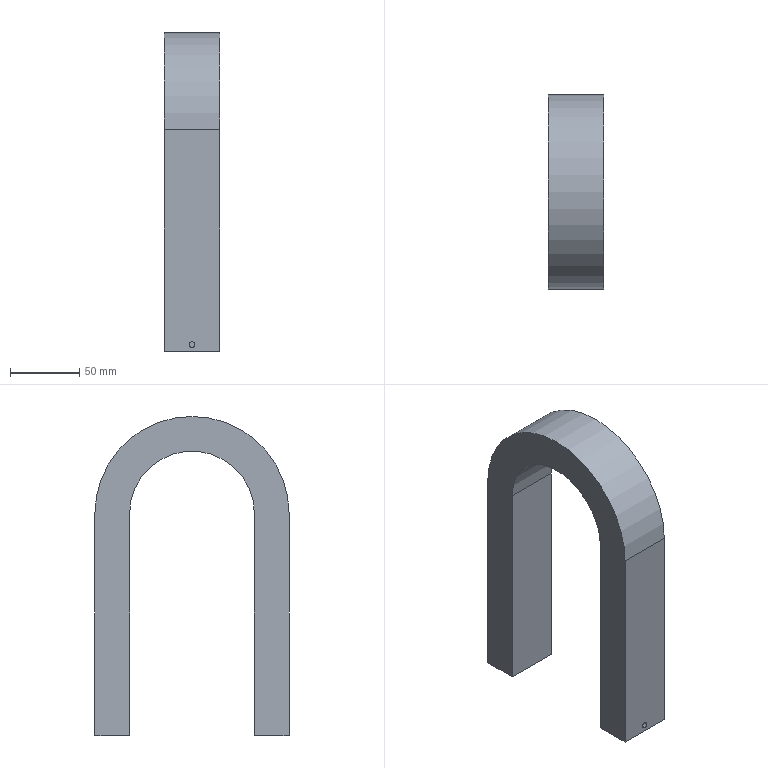Part | STEP file | material-separating mechanism drag chain | 1 solid | 12 faces | box 40 x 140 x 230 mm | volume 500295 mm3 | plane 8 | cylinder 4 | commonest cylinder face diameters 4.2 x2 90 x1 140 x1
STEP:
#1=CARTESIAN_POINT('',(0.,0.,0.));
#2=DIRECTION('',(0.,0.,1.));
#3=DIRECTION('',(1.,0.,0.));
#4=AXIS2_PLACEMENT_3D('',#1,#2,#3);
#5=CARTESIAN_POINT('',(5.,0.,7.1));
#6=VERTEX_POINT('',#5);
#7=CARTESIAN_POINT('',(5.,25.,7.1));
#8=VERTEX_POINT('',#7);
#9=CARTESIAN_POINT('',(5.,25.,7.1));
#10=DIRECTION('',(0.,1.,0.));
#11=VECTOR('',#10,1.);
#12=LINE('',#9,#11);
#13=CARTESIAN_POINT('',(5.,25.,5.));
#14=DIRECTION('',(0.,1.,0.));
#15=DIRECTION('',(0.,0.,1.));
#16=AXIS2_PLACEMENT_3D('',#13,#14,#15);
#17=CYLINDRICAL_SURFACE('',#16,2.1);
#18=CARTESIAN_POINT('',(6.283,0.));
#19=DIRECTION('',(0.,1.));
#20=VECTOR('',#19,1.);
#21=LINE('',#18,#20);
#22=(GEOMETRIC_REPRESENTATION_CONTEXT(2)PARAMETRIC_REPRESENTATION_CONTEXT()REPRESENTATION_CONTEXT('',''));
#23=DEFINITIONAL_REPRESENTATION('',(#21),#22);
#24=PCURVE('',#17,#23);
#25=CARTESIAN_POINT('',(5.,25.,5.));
#26=DIRECTION('',(0.,1.,0.));
#27=DIRECTION('',(0.,0.,1.));
#28=AXIS2_PLACEMENT_3D('',#25,#26,#27);
#29=CYLINDRICAL_SURFACE('',#28,2.1);
#30=CARTESIAN_POINT('',(0.,0.));
#31=DIRECTION('',(0.,1.));
#32=VECTOR('',#31,1.);
#33=LINE('',#30,#32);
#34=(GEOMETRIC_REPRESENTATION_CONTEXT(2)PARAMETRIC_REPRESENTATION_CONTEXT()REPRESENTATION_CONTEXT('',''));
#35=DEFINITIONAL_REPRESENTATION('',(#33),#34);
#36=PCURVE('',#29,#35);
#37=SURFACE_CURVE('',#12,(#24,#36),.PCURVE_S1.);
#38=EDGE_CURVE('',#6,#8,#37,.T.);
#39=ORIENTED_EDGE('',*,*,#38,.T.);
#40=CARTESIAN_POINT('',(5.,25.,2.9));
#41=VERTEX_POINT('',#40);
#42=CARTESIAN_POINT('',(5.,25.,5.));
#43=DIRECTION('',(0.,1.,0.));
#44=DIRECTION('',(0.,0.,1.));
#45=AXIS2_PLACEMENT_3D('',#42,#43,#44);
#46=CIRCLE('',#45,2.1);
#47=CARTESIAN_POINT('',(0.,0.));
#48=DIRECTION('',(1.,0.));
#49=VECTOR('',#48,1.);
#50=LINE('',#47,#49);
#51=(GEOMETRIC_REPRESENTATION_CONTEXT(2)PARAMETRIC_REPRESENTATION_CONTEXT()REPRESENTATION_CONTEXT('',''));
#52=DEFINITIONAL_REPRESENTATION('',(#50),#51);
#53=PCURVE('',#17,#52);
#54=CARTESIAN_POINT('',(-15.,25.,0.));
#55=DIRECTION('',(0.,1.,0.));
#56=DIRECTION('',(0.,0.,1.));
#57=AXIS2_PLACEMENT_3D('',#54,#55,#56);
#58=PLANE('',#57);
#59=CARTESIAN_POINT('',(5.,20.));
#60=DIRECTION('',(1.,0.));
#61=AXIS2_PLACEMENT_2D('',#59,#60);
#62=CIRCLE('',#61,2.1);
#63=(GEOMETRIC_REPRESENTATION_CONTEXT(2)PARAMETRIC_REPRESENTATION_CONTEXT()REPRESENTATION_CONTEXT('',''));
#64=DEFINITIONAL_REPRESENTATION('',(#62),#63);
#65=PCURVE('',#58,#64);
#66=SURFACE_CURVE('',#46,(#53,#65),.PCURVE_S1.);
#67=EDGE_CURVE('',#41,#8,#66,.T.);
#68=ORIENTED_EDGE('',*,*,#67,.F.);
#69=CARTESIAN_POINT('',(5.,0.,2.9));
#70=VERTEX_POINT('',#69);
#71=CARTESIAN_POINT('',(5.,25.,2.9));
#72=DIRECTION('',(0.,1.,0.));
#73=VECTOR('',#72,1.);
#74=LINE('',#71,#73);
#75=CARTESIAN_POINT('',(3.142,0.));
#76=DIRECTION('',(0.,1.));
#77=VECTOR('',#76,1.);
#78=LINE('',#75,#77);
#79=(GEOMETRIC_REPRESENTATION_CONTEXT(2)PARAMETRIC_REPRESENTATION_CONTEXT()REPRESENTATION_CONTEXT('',''));
#80=DEFINITIONAL_REPRESENTATION('',(#78),#79);
#81=PCURVE('',#17,#80);
#82=CARTESIAN_POINT('',(3.142,0.));
#83=DIRECTION('',(0.,1.));
#84=VECTOR('',#83,1.);
#85=LINE('',#82,#84);
#86=(GEOMETRIC_REPRESENTATION_CONTEXT(2)PARAMETRIC_REPRESENTATION_CONTEXT()REPRESENTATION_CONTEXT('',''));
#87=DEFINITIONAL_REPRESENTATION('',(#85),#86);
#88=PCURVE('',#29,#87);
#89=SURFACE_CURVE('',#74,(#81,#88),.PCURVE_S1.);
#90=EDGE_CURVE('',#70,#41,#89,.T.);
#91=ORIENTED_EDGE('',*,*,#90,.F.);
#92=CARTESIAN_POINT('',(5.,0.,5.));
#93=DIRECTION('',(0.,1.,0.));
#94=DIRECTION('',(0.,0.,1.));
#95=AXIS2_PLACEMENT_3D('',#92,#93,#94);
#96=CIRCLE('',#95,2.1);
#97=CARTESIAN_POINT('',(0.,-25.));
#98=DIRECTION('',(1.,0.));
#99=VECTOR('',#98,1.);
#100=LINE('',#97,#99);
#101=(GEOMETRIC_REPRESENTATION_CONTEXT(2)PARAMETRIC_REPRESENTATION_CONTEXT()REPRESENTATION_CONTEXT('',''));
#102=DEFINITIONAL_REPRESENTATION('',(#100),#101);
#103=PCURVE('',#17,#102);
#104=CARTESIAN_POINT('',(-15.,0.,0.));
#105=DIRECTION('',(0.,-1.,0.));
#106=DIRECTION('',(0.,0.,-1.));
#107=AXIS2_PLACEMENT_3D('',#104,#105,#106);
#108=PLANE('',#107);
#109=CARTESIAN_POINT('',(-7.1,20.));
#110=CARTESIAN_POINT('',(-7.1,23.637));
#111=CARTESIAN_POINT('',(-3.95,21.819));
#112=CARTESIAN_POINT('',(-0.8,20.));
#113=CARTESIAN_POINT('',(-3.95,18.181));
#114=CARTESIAN_POINT('',(-7.1,16.363));
#115=CARTESIAN_POINT('',(-7.1,20.));
#116=(BOUNDED_CURVE()B_SPLINE_CURVE(2,(#109,#110,#111,#112,#113,#114,#115),.UNSPECIFIED.,.T.,.F.)B_SPLINE_CURVE_WITH_KNOTS((1,2,2,2,2,1),(-2.094,0.,2.094,4.189,6.283,8.378),.UNSPECIFIED.)CURVE()GEOMETRIC_REPRESENTATION_ITEM()RATIONAL_B_SPLINE_CURVE((1.,0.5,1.,0.5,1.,0.5,1.))REPRESENTATION_ITEM(''));
#117=(GEOMETRIC_REPRESENTATION_CONTEXT(2)PARAMETRIC_REPRESENTATION_CONTEXT()REPRESENTATION_CONTEXT('',''));
#118=DEFINITIONAL_REPRESENTATION('',(#116),#117);
#119=PCURVE('',#108,#118);
#120=SURFACE_CURVE('',#96,(#103,#119),.PCURVE_S1.);
#121=EDGE_CURVE('',#70,#6,#120,.T.);
#122=ORIENTED_EDGE('',*,*,#121,.T.);
#123=EDGE_LOOP('',(#39,#68,#91,#122));
#124=FACE_BOUND('',#123,.F.);
#125=ADVANCED_FACE('',(#124),#17,.F.);
#126=CARTESIAN_POINT('',(-15.,0.,160.));
#127=VERTEX_POINT('',#126);
#128=CARTESIAN_POINT('',(25.,0.,160.));
#129=VERTEX_POINT('',#128);
#130=CARTESIAN_POINT('',(-15.,0.,160.));
#131=DIRECTION('',(1.,0.,0.));
#132=VECTOR('',#131,1.);
#133=LINE('',#130,#132);
#134=CARTESIAN_POINT('',(-15.,70.,160.));
#135=DIRECTION('',(1.,0.,0.));
#136=DIRECTION('',(0.,0.,-1.));
#137=AXIS2_PLACEMENT_3D('',#134,#135,#136);
#138=CYLINDRICAL_SURFACE('',#137,70.);
#139=CARTESIAN_POINT('',(4.712,0.));
#140=DIRECTION('',(0.,1.));
#141=VECTOR('',#140,1.);
#142=LINE('',#139,#141);
#143=(GEOMETRIC_REPRESENTATION_CONTEXT(2)PARAMETRIC_REPRESENTATION_CONTEXT()REPRESENTATION_CONTEXT('',''));
#144=DEFINITIONAL_REPRESENTATION('',(#142),#143);
#145=PCURVE('',#138,#144);
#146=CARTESIAN_POINT('',(-160.,0.));
#147=DIRECTION('',(0.,1.));
#148=VECTOR('',#147,1.);
#149=LINE('',#146,#148);
#150=(GEOMETRIC_REPRESENTATION_CONTEXT(2)PARAMETRIC_REPRESENTATION_CONTEXT()REPRESENTATION_CONTEXT('',''));
#151=DEFINITIONAL_REPRESENTATION('',(#149),#150);
#152=PCURVE('',#108,#151);
#153=SURFACE_CURVE('',#133,(#145,#152),.PCURVE_S1.);
#154=EDGE_CURVE('',#127,#129,#153,.T.);
#155=ORIENTED_EDGE('',*,*,#154,.T.);
#156=CARTESIAN_POINT('',(25.,140.,160.));
#157=VERTEX_POINT('',#156);
#158=CARTESIAN_POINT('',(25.,70.,160.));
#159=DIRECTION('',(1.,0.,0.));
#160=DIRECTION('',(0.,0.,-1.));
#161=AXIS2_PLACEMENT_3D('',#158,#159,#160);
#162=CIRCLE('',#161,70.);
#163=CARTESIAN_POINT('',(0.,40.));
#164=DIRECTION('',(1.,0.));
#165=VECTOR('',#164,1.);
#166=LINE('',#163,#165);
#167=(GEOMETRIC_REPRESENTATION_CONTEXT(2)PARAMETRIC_REPRESENTATION_CONTEXT()REPRESENTATION_CONTEXT('',''));
#168=DEFINITIONAL_REPRESENTATION('',(#166),#167);
#169=PCURVE('',#138,#168);
#170=CARTESIAN_POINT('',(25.,70.,160.));
#171=DIRECTION('',(1.,0.,0.));
#172=DIRECTION('',(0.,0.,-1.));
#173=AXIS2_PLACEMENT_3D('',#170,#171,#172);
#174=PLANE('',#173);
#175=CARTESIAN_POINT('',(0.,0.));
#176=DIRECTION('',(1.,0.));
#177=AXIS2_PLACEMENT_2D('',#175,#176);
#178=CIRCLE('',#177,70.);
#179=(GEOMETRIC_REPRESENTATION_CONTEXT(2)PARAMETRIC_REPRESENTATION_CONTEXT()REPRESENTATION_CONTEXT('',''));
#180=DEFINITIONAL_REPRESENTATION('',(#178),#179);
#181=PCURVE('',#174,#180);
#182=SURFACE_CURVE('',#162,(#169,#181),.PCURVE_S1.);
#183=EDGE_CURVE('',#157,#129,#182,.T.);
#184=ORIENTED_EDGE('',*,*,#183,.F.);
#185=CARTESIAN_POINT('',(-15.,140.,160.));
#186=VERTEX_POINT('',#185);
#187=CARTESIAN_POINT('',(-15.,140.,160.));
#188=DIRECTION('',(1.,0.,0.));
#189=VECTOR('',#188,1.);
#190=LINE('',#187,#189);
#191=CARTESIAN_POINT('',(1.571,0.));
#192=DIRECTION('',(0.,1.));
#193=VECTOR('',#192,1.);
#194=LINE('',#191,#193);
#195=(GEOMETRIC_REPRESENTATION_CONTEXT(2)PARAMETRIC_REPRESENTATION_CONTEXT()REPRESENTATION_CONTEXT('',''));
#196=DEFINITIONAL_REPRESENTATION('',(#194),#195);
#197=PCURVE('',#138,#196);
#198=CARTESIAN_POINT('',(-15.,140.,0.));
#199=DIRECTION('',(0.,1.,0.));
#200=DIRECTION('',(0.,0.,1.));
#201=AXIS2_PLACEMENT_3D('',#198,#199,#200);
#202=PLANE('',#201);
#203=CARTESIAN_POINT('',(160.,0.));
#204=DIRECTION('',(0.,1.));
#205=VECTOR('',#204,1.);
#206=LINE('',#203,#205);
#207=(GEOMETRIC_REPRESENTATION_CONTEXT(2)PARAMETRIC_REPRESENTATION_CONTEXT()REPRESENTATION_CONTEXT('',''));
#208=DEFINITIONAL_REPRESENTATION('',(#206),#207);
#209=PCURVE('',#202,#208);
#210=SURFACE_CURVE('',#190,(#197,#209),.PCURVE_S1.);
#211=EDGE_CURVE('',#186,#157,#210,.T.);
#212=ORIENTED_EDGE('',*,*,#211,.F.);
#213=CARTESIAN_POINT('',(-15.,70.,160.));
#214=DIRECTION('',(1.,0.,0.));
#215=DIRECTION('',(0.,0.,-1.));
#216=AXIS2_PLACEMENT_3D('',#213,#214,#215);
#217=CIRCLE('',#216,70.);
#218=CARTESIAN_POINT('',(0.,0.));
#219=DIRECTION('',(1.,0.));
#220=VECTOR('',#219,1.);
#221=LINE('',#218,#220);
#222=(GEOMETRIC_REPRESENTATION_CONTEXT(2)PARAMETRIC_REPRESENTATION_CONTEXT()REPRESENTATION_CONTEXT('',''));
#223=DEFINITIONAL_REPRESENTATION('',(#221),#222);
#224=PCURVE('',#138,#223);
#225=CARTESIAN_POINT('',(-15.,70.,160.));
#226=DIRECTION('',(1.,0.,0.));
#227=DIRECTION('',(0.,0.,-1.));
#228=AXIS2_PLACEMENT_3D('',#225,#226,#227);
#229=PLANE('',#228);
#230=CARTESIAN_POINT('',(0.,0.));
#231=DIRECTION('',(1.,0.));
#232=AXIS2_PLACEMENT_2D('',#230,#231);
#233=CIRCLE('',#232,70.);
#234=(GEOMETRIC_REPRESENTATION_CONTEXT(2)PARAMETRIC_REPRESENTATION_CONTEXT()REPRESENTATION_CONTEXT('',''));
#235=DEFINITIONAL_REPRESENTATION('',(#233),#234);
#236=PCURVE('',#229,#235);
#237=SURFACE_CURVE('',#217,(#224,#236),.PCURVE_S1.);
#238=EDGE_CURVE('',#186,#127,#237,.T.);
#239=ORIENTED_EDGE('',*,*,#238,.T.);
#240=EDGE_LOOP('',(#155,#184,#212,#239));
#241=FACE_BOUND('',#240,.T.);
#242=ADVANCED_FACE('',(#241),#138,.T.);
#243=ORIENTED_EDGE('',*,*,#211,.T.);
#244=CARTESIAN_POINT('',(25.,140.,0.));
#245=VERTEX_POINT('',#244);
#246=CARTESIAN_POINT('',(25.,140.,0.));
#247=DIRECTION('',(0.,0.,1.));
#248=VECTOR('',#247,1.);
#249=LINE('',#246,#248);
#250=CARTESIAN_POINT('',(0.,40.));
#251=DIRECTION('',(1.,0.));
#252=VECTOR('',#251,1.);
#253=LINE('',#250,#252);
#254=(GEOMETRIC_REPRESENTATION_CONTEXT(2)PARAMETRIC_REPRESENTATION_CONTEXT()REPRESENTATION_CONTEXT('',''));
#255=DEFINITIONAL_REPRESENTATION('',(#253),#254);
#256=PCURVE('',#202,#255);
#257=CARTESIAN_POINT('',(160.,70.));
#258=DIRECTION('',(-1.,0.));
#259=VECTOR('',#258,1.);
#260=LINE('',#257,#259);
#261=(GEOMETRIC_REPRESENTATION_CONTEXT(2)PARAMETRIC_REPRESENTATION_CONTEXT()REPRESENTATION_CONTEXT('',''));
#262=DEFINITIONAL_REPRESENTATION('',(#260),#261);
#263=PCURVE('',#174,#262);
#264=SURFACE_CURVE('',#249,(#256,#263),.PCURVE_S1.);
#265=EDGE_CURVE('',#245,#157,#264,.T.);
#266=ORIENTED_EDGE('',*,*,#265,.F.);
#267=CARTESIAN_POINT('',(-15.,140.,0.));
#268=VERTEX_POINT('',#267);
#269=CARTESIAN_POINT('',(-15.,140.,0.));
#270=DIRECTION('',(1.,0.,0.));
#271=VECTOR('',#270,1.);
#272=LINE('',#269,#271);
#273=CARTESIAN_POINT('',(0.,0.));
#274=DIRECTION('',(0.,1.));
#275=VECTOR('',#274,1.);
#276=LINE('',#273,#275);
#277=(GEOMETRIC_REPRESENTATION_CONTEXT(2)PARAMETRIC_REPRESENTATION_CONTEXT()REPRESENTATION_CONTEXT('',''));
#278=DEFINITIONAL_REPRESENTATION('',(#276),#277);
#279=PCURVE('',#202,#278);
#280=CARTESIAN_POINT('',(-15.,140.,0.));
#281=DIRECTION('',(0.,0.,-1.));
#282=DIRECTION('',(0.,1.,0.));
#283=AXIS2_PLACEMENT_3D('',#280,#281,#282);
#284=PLANE('',#283);
#285=CARTESIAN_POINT('',(0.,0.));
#286=DIRECTION('',(0.,1.));
#287=VECTOR('',#286,1.);
#288=LINE('',#285,#287);
#289=(GEOMETRIC_REPRESENTATION_CONTEXT(2)PARAMETRIC_REPRESENTATION_CONTEXT()REPRESENTATION_CONTEXT('',''));
#290=DEFINITIONAL_REPRESENTATION('',(#288),#289);
#291=PCURVE('',#284,#290);
#292=SURFACE_CURVE('',#272,(#279,#291),.PCURVE_S1.);
#293=EDGE_CURVE('',#268,#245,#292,.T.);
#294=ORIENTED_EDGE('',*,*,#293,.F.);
#295=CARTESIAN_POINT('',(-15.,140.,0.));
#296=DIRECTION('',(0.,0.,1.));
#297=VECTOR('',#296,1.);
#298=LINE('',#295,#297);
#299=CARTESIAN_POINT('',(0.,0.));
#300=DIRECTION('',(1.,0.));
#301=VECTOR('',#300,1.);
#302=LINE('',#299,#301);
#303=(GEOMETRIC_REPRESENTATION_CONTEXT(2)PARAMETRIC_REPRESENTATION_CONTEXT()REPRESENTATION_CONTEXT('',''));
#304=DEFINITIONAL_REPRESENTATION('',(#302),#303);
#305=PCURVE('',#202,#304);
#306=CARTESIAN_POINT('',(160.,70.));
#307=DIRECTION('',(-1.,0.));
#308=VECTOR('',#307,1.);
#309=LINE('',#306,#308);
#310=(GEOMETRIC_REPRESENTATION_CONTEXT(2)PARAMETRIC_REPRESENTATION_CONTEXT()REPRESENTATION_CONTEXT('',''));
#311=DEFINITIONAL_REPRESENTATION('',(#309),#310);
#312=PCURVE('',#229,#311);
#313=SURFACE_CURVE('',#298,(#305,#312),.PCURVE_S1.);
#314=EDGE_CURVE('',#268,#186,#313,.T.);
#315=ORIENTED_EDGE('',*,*,#314,.T.);
#316=EDGE_LOOP('',(#243,#266,#294,#315));
#317=FACE_BOUND('',#316,.T.);
#318=ADVANCED_FACE('',(#317),#202,.T.);
#319=ORIENTED_EDGE('',*,*,#293,.T.);
#320=CARTESIAN_POINT('',(25.,115.,0.));
#321=VERTEX_POINT('',#320);
#322=CARTESIAN_POINT('',(25.,140.,0.));
#323=DIRECTION('',(0.,1.,0.));
#324=VECTOR('',#323,1.);
#325=LINE('',#322,#324);
#326=CARTESIAN_POINT('',(0.,40.));
#327=DIRECTION('',(1.,0.));
#328=VECTOR('',#327,1.);
#329=LINE('',#326,#328);
#330=(GEOMETRIC_REPRESENTATION_CONTEXT(2)PARAMETRIC_REPRESENTATION_CONTEXT()REPRESENTATION_CONTEXT('',''));
#331=DEFINITIONAL_REPRESENTATION('',(#329),#330);
#332=PCURVE('',#284,#331);
#333=CARTESIAN_POINT('',(160.,70.));
#334=DIRECTION('',(0.,1.));
#335=VECTOR('',#334,1.);
#336=LINE('',#333,#335);
#337=(GEOMETRIC_REPRESENTATION_CONTEXT(2)PARAMETRIC_REPRESENTATION_CONTEXT()REPRESENTATION_CONTEXT('',''));
#338=DEFINITIONAL_REPRESENTATION('',(#336),#337);
#339=PCURVE('',#174,#338);
#340=SURFACE_CURVE('',#325,(#332,#339),.PCURVE_S1.);
#341=EDGE_CURVE('',#321,#245,#340,.T.);
#342=ORIENTED_EDGE('',*,*,#341,.F.);
#343=CARTESIAN_POINT('',(-15.,115.,0.));
#344=VERTEX_POINT('',#343);
#345=CARTESIAN_POINT('',(-15.,115.,0.));
#346=DIRECTION('',(1.,0.,0.));
#347=VECTOR('',#346,1.);
#348=LINE('',#345,#347);
#349=CARTESIAN_POINT('',(-25.,0.));
#350=DIRECTION('',(0.,1.));
#351=VECTOR('',#350,1.);
#352=LINE('',#349,#351);
#353=(GEOMETRIC_REPRESENTATION_CONTEXT(2)PARAMETRIC_REPRESENTATION_CONTEXT()REPRESENTATION_CONTEXT('',''));
#354=DEFINITIONAL_REPRESENTATION('',(#352),#353);
#355=PCURVE('',#284,#354);
#356=CARTESIAN_POINT('',(-15.,115.,0.));
#357=DIRECTION('',(0.,-1.,0.));
#358=DIRECTION('',(0.,0.,-1.));
#359=AXIS2_PLACEMENT_3D('',#356,#357,#358);
#360=PLANE('',#359);
#361=CARTESIAN_POINT('',(0.,0.));
#362=DIRECTION('',(0.,1.));
#363=VECTOR('',#362,1.);
#364=LINE('',#361,#363);
#365=(GEOMETRIC_REPRESENTATION_CONTEXT(2)PARAMETRIC_REPRESENTATION_CONTEXT()REPRESENTATION_CONTEXT('',''));
#366=DEFINITIONAL_REPRESENTATION('',(#364),#365);
#367=PCURVE('',#360,#366);
#368=SURFACE_CURVE('',#348,(#355,#367),.PCURVE_S1.);
#369=EDGE_CURVE('',#344,#321,#368,.T.);
#370=ORIENTED_EDGE('',*,*,#369,.F.);
#371=CARTESIAN_POINT('',(-15.,140.,0.));
#372=DIRECTION('',(0.,1.,0.));
#373=VECTOR('',#372,1.);
#374=LINE('',#371,#373);
#375=CARTESIAN_POINT('',(0.,0.));
#376=DIRECTION('',(1.,0.));
#377=VECTOR('',#376,1.);
#378=LINE('',#375,#377);
#379=(GEOMETRIC_REPRESENTATION_CONTEXT(2)PARAMETRIC_REPRESENTATION_CONTEXT()REPRESENTATION_CONTEXT('',''));
#380=DEFINITIONAL_REPRESENTATION('',(#378),#379);
#381=PCURVE('',#284,#380);
#382=CARTESIAN_POINT('',(160.,70.));
#383=DIRECTION('',(0.,1.));
#384=VECTOR('',#383,1.);
#385=LINE('',#382,#384);
#386=(GEOMETRIC_REPRESENTATION_CONTEXT(2)PARAMETRIC_REPRESENTATION_CONTEXT()REPRESENTATION_CONTEXT('',''));
#387=DEFINITIONAL_REPRESENTATION('',(#385),#386);
#388=PCURVE('',#229,#387);
#389=SURFACE_CURVE('',#374,(#381,#388),.PCURVE_S1.);
#390=EDGE_CURVE('',#344,#268,#389,.T.);
#391=ORIENTED_EDGE('',*,*,#390,.T.);
#392=EDGE_LOOP('',(#319,#342,#370,#391));
#393=FACE_BOUND('',#392,.T.);
#394=ADVANCED_FACE('',(#393),#284,.T.);
#395=ORIENTED_EDGE('',*,*,#369,.T.);
#396=CARTESIAN_POINT('',(25.,115.,160.));
#397=VERTEX_POINT('',#396);
#398=CARTESIAN_POINT('',(25.,115.,0.));
#399=DIRECTION('',(0.,0.,-1.));
#400=VECTOR('',#399,1.);
#401=LINE('',#398,#400);
#402=CARTESIAN_POINT('',(0.,40.));
#403=DIRECTION('',(1.,0.));
#404=VECTOR('',#403,1.);
#405=LINE('',#402,#404);
#406=(GEOMETRIC_REPRESENTATION_CONTEXT(2)PARAMETRIC_REPRESENTATION_CONTEXT()REPRESENTATION_CONTEXT('',''));
#407=DEFINITIONAL_REPRESENTATION('',(#405),#406);
#408=PCURVE('',#360,#407);
#409=CARTESIAN_POINT('',(160.,45.));
#410=DIRECTION('',(1.,0.));
#411=VECTOR('',#410,1.);
#412=LINE('',#409,#411);
#413=(GEOMETRIC_REPRESENTATION_CONTEXT(2)PARAMETRIC_REPRESENTATION_CONTEXT()REPRESENTATION_CONTEXT('',''));
#414=DEFINITIONAL_REPRESENTATION('',(#412),#413);
#415=PCURVE('',#174,#414);
#416=SURFACE_CURVE('',#401,(#408,#415),.PCURVE_S1.);
#417=EDGE_CURVE('',#397,#321,#416,.T.);
#418=ORIENTED_EDGE('',*,*,#417,.F.);
#419=CARTESIAN_POINT('',(-15.,115.,160.));
#420=VERTEX_POINT('',#419);
#421=CARTESIAN_POINT('',(-15.,115.,160.));
#422=DIRECTION('',(1.,0.,0.));
#423=VECTOR('',#422,1.);
#424=LINE('',#421,#423);
#425=CARTESIAN_POINT('',(-160.,0.));
#426=DIRECTION('',(0.,1.));
#427=VECTOR('',#426,1.);
#428=LINE('',#425,#427);
#429=(GEOMETRIC_REPRESENTATION_CONTEXT(2)PARAMETRIC_REPRESENTATION_CONTEXT()REPRESENTATION_CONTEXT('',''));
#430=DEFINITIONAL_REPRESENTATION('',(#428),#429);
#431=PCURVE('',#360,#430);
#432=CARTESIAN_POINT('',(-15.,70.,160.));
#433=DIRECTION('',(1.,0.,0.));
#434=DIRECTION('',(0.,0.,-1.));
#435=AXIS2_PLACEMENT_3D('',#432,#433,#434);
#436=CYLINDRICAL_SURFACE('',#435,45.);
#437=CARTESIAN_POINT('',(1.571,0.));
#438=DIRECTION('',(0.,1.));
#439=VECTOR('',#438,1.);
#440=LINE('',#437,#439);
#441=(GEOMETRIC_REPRESENTATION_CONTEXT(2)PARAMETRIC_REPRESENTATION_CONTEXT()REPRESENTATION_CONTEXT('',''));
#442=DEFINITIONAL_REPRESENTATION('',(#440),#441);
#443=PCURVE('',#436,#442);
#444=SURFACE_CURVE('',#424,(#431,#443),.PCURVE_S1.);
#445=EDGE_CURVE('',#420,#397,#444,.T.);
#446=ORIENTED_EDGE('',*,*,#445,.F.);
#447=CARTESIAN_POINT('',(-15.,115.,0.));
#448=DIRECTION('',(0.,0.,-1.));
#449=VECTOR('',#448,1.);
#450=LINE('',#447,#449);
#451=CARTESIAN_POINT('',(0.,0.));
#452=DIRECTION('',(1.,0.));
#453=VECTOR('',#452,1.);
#454=LINE('',#451,#453);
#455=(GEOMETRIC_REPRESENTATION_CONTEXT(2)PARAMETRIC_REPRESENTATION_CONTEXT()REPRESENTATION_CONTEXT('',''));
#456=DEFINITIONAL_REPRESENTATION('',(#454),#455);
#457=PCURVE('',#360,#456);
#458=CARTESIAN_POINT('',(160.,45.));
#459=DIRECTION('',(1.,0.));
#460=VECTOR('',#459,1.);
#461=LINE('',#458,#460);
#462=(GEOMETRIC_REPRESENTATION_CONTEXT(2)PARAMETRIC_REPRESENTATION_CONTEXT()REPRESENTATION_CONTEXT('',''));
#463=DEFINITIONAL_REPRESENTATION('',(#461),#462);
#464=PCURVE('',#229,#463);
#465=SURFACE_CURVE('',#450,(#457,#464),.PCURVE_S1.);
#466=EDGE_CURVE('',#420,#344,#465,.T.);
#467=ORIENTED_EDGE('',*,*,#466,.T.);
#468=EDGE_LOOP('',(#395,#418,#446,#467));
#469=FACE_BOUND('',#468,.T.);
#470=ADVANCED_FACE('',(#469),#360,.T.);
#471=CARTESIAN_POINT('',(-15.,25.,160.));
#472=VERTEX_POINT('',#471);
#473=CARTESIAN_POINT('',(-15.,70.,160.));
#474=DIRECTION('',(-1.,0.,0.));
#475=DIRECTION('',(0.,0.,-1.));
#476=AXIS2_PLACEMENT_3D('',#473,#474,#475);
#477=CIRCLE('',#476,45.);
#478=CARTESIAN_POINT('',(6.283,0.));
#479=DIRECTION('',(-1.,0.));
#480=VECTOR('',#479,1.);
#481=LINE('',#478,#480);
#482=(GEOMETRIC_REPRESENTATION_CONTEXT(2)PARAMETRIC_REPRESENTATION_CONTEXT()REPRESENTATION_CONTEXT('',''));
#483=DEFINITIONAL_REPRESENTATION('',(#481),#482);
#484=PCURVE('',#436,#483);
#485=CARTESIAN_POINT('',(45.,0.));
#486=CARTESIAN_POINT('',(45.,-77.942));
#487=CARTESIAN_POINT('',(-22.5,-38.971));
#488=CARTESIAN_POINT('',(-90.,0.));
#489=CARTESIAN_POINT('',(-22.5,38.971));
#490=CARTESIAN_POINT('',(45.,77.942));
#491=CARTESIAN_POINT('',(45.,0.));
#492=(BOUNDED_CURVE()B_SPLINE_CURVE(2,(#485,#486,#487,#488,#489,#490,#491),.UNSPECIFIED.,.T.,.F.)B_SPLINE_CURVE_WITH_KNOTS((1,2,2,2,2,1),(-2.094,0.,2.094,4.189,6.283,8.378),.UNSPECIFIED.)CURVE()GEOMETRIC_REPRESENTATION_ITEM()RATIONAL_B_SPLINE_CURVE((1.,0.5,1.,0.5,1.,0.5,1.))REPRESENTATION_ITEM(''));
#493=(GEOMETRIC_REPRESENTATION_CONTEXT(2)PARAMETRIC_REPRESENTATION_CONTEXT()REPRESENTATION_CONTEXT('',''));
#494=DEFINITIONAL_REPRESENTATION('',(#492),#493);
#495=PCURVE('',#229,#494);
#496=SURFACE_CURVE('',#477,(#484,#495),.PCURVE_S1.);
#497=EDGE_CURVE('',#472,#420,#496,.T.);
#498=ORIENTED_EDGE('',*,*,#497,.F.);
#499=CARTESIAN_POINT('',(25.,25.,160.));
#500=VERTEX_POINT('',#499);
#501=CARTESIAN_POINT('',(-15.,25.,160.));
#502=DIRECTION('',(1.,0.,0.));
#503=VECTOR('',#502,1.);
#504=LINE('',#501,#503);
#505=CARTESIAN_POINT('',(4.712,0.));
#506=DIRECTION('',(0.,1.));
#507=VECTOR('',#506,1.);
#508=LINE('',#505,#507);
#509=(GEOMETRIC_REPRESENTATION_CONTEXT(2)PARAMETRIC_REPRESENTATION_CONTEXT()REPRESENTATION_CONTEXT('',''));
#510=DEFINITIONAL_REPRESENTATION('',(#508),#509);
#511=PCURVE('',#436,#510);
#512=CARTESIAN_POINT('',(160.,0.));
#513=DIRECTION('',(0.,1.));
#514=VECTOR('',#513,1.);
#515=LINE('',#512,#514);
#516=(GEOMETRIC_REPRESENTATION_CONTEXT(2)PARAMETRIC_REPRESENTATION_CONTEXT()REPRESENTATION_CONTEXT('',''));
#517=DEFINITIONAL_REPRESENTATION('',(#515),#516);
#518=PCURVE('',#58,#517);
#519=SURFACE_CURVE('',#504,(#511,#518),.PCURVE_S1.);
#520=EDGE_CURVE('',#472,#500,#519,.T.);
#521=ORIENTED_EDGE('',*,*,#520,.T.);
#522=CARTESIAN_POINT('',(25.,70.,160.));
#523=DIRECTION('',(-1.,0.,0.));
#524=DIRECTION('',(0.,0.,-1.));
#525=AXIS2_PLACEMENT_3D('',#522,#523,#524);
#526=CIRCLE('',#525,45.);
#527=CARTESIAN_POINT('',(6.283,40.));
#528=DIRECTION('',(-1.,0.));
#529=VECTOR('',#528,1.);
#530=LINE('',#527,#529);
#531=(GEOMETRIC_REPRESENTATION_CONTEXT(2)PARAMETRIC_REPRESENTATION_CONTEXT()REPRESENTATION_CONTEXT('',''));
#532=DEFINITIONAL_REPRESENTATION('',(#530),#531);
#533=PCURVE('',#436,#532);
#534=CARTESIAN_POINT('',(45.,0.));
#535=CARTESIAN_POINT('',(45.,-77.942));
#536=CARTESIAN_POINT('',(-22.5,-38.971));
#537=CARTESIAN_POINT('',(-90.,0.));
#538=CARTESIAN_POINT('',(-22.5,38.971));
#539=CARTESIAN_POINT('',(45.,77.942));
#540=CARTESIAN_POINT('',(45.,0.));
#541=(BOUNDED_CURVE()B_SPLINE_CURVE(2,(#534,#535,#536,#537,#538,#539,#540),.UNSPECIFIED.,.T.,.F.)B_SPLINE_CURVE_WITH_KNOTS((1,2,2,2,2,1),(-2.094,0.,2.094,4.189,6.283,8.378),.UNSPECIFIED.)CURVE()GEOMETRIC_REPRESENTATION_ITEM()RATIONAL_B_SPLINE_CURVE((1.,0.5,1.,0.5,1.,0.5,1.))REPRESENTATION_ITEM(''));
#542=(GEOMETRIC_REPRESENTATION_CONTEXT(2)PARAMETRIC_REPRESENTATION_CONTEXT()REPRESENTATION_CONTEXT('',''));
#543=DEFINITIONAL_REPRESENTATION('',(#541),#542);
#544=PCURVE('',#174,#543);
#545=SURFACE_CURVE('',#526,(#533,#544),.PCURVE_S1.);
#546=EDGE_CURVE('',#500,#397,#545,.T.);
#547=ORIENTED_EDGE('',*,*,#546,.T.);
#548=ORIENTED_EDGE('',*,*,#445,.F.);
#549=EDGE_LOOP('',(#498,#521,#547,#548));
#550=FACE_BOUND('',#549,.F.);
#551=ADVANCED_FACE('',(#550),#436,.F.);
#552=CARTESIAN_POINT('',(5.,25.,5.));
#553=DIRECTION('',(0.,1.,0.));
#554=DIRECTION('',(0.,0.,1.));
#555=AXIS2_PLACEMENT_3D('',#552,#553,#554);
#556=CIRCLE('',#555,2.1);
#557=CARTESIAN_POINT('',(5.,20.));
#558=DIRECTION('',(1.,0.));
#559=AXIS2_PLACEMENT_2D('',#557,#558);
#560=CIRCLE('',#559,2.1);
#561=(GEOMETRIC_REPRESENTATION_CONTEXT(2)PARAMETRIC_REPRESENTATION_CONTEXT()REPRESENTATION_CONTEXT('',''));
#562=DEFINITIONAL_REPRESENTATION('',(#560),#561);
#563=PCURVE('',#58,#562);
#564=CARTESIAN_POINT('',(0.,0.));
#565=DIRECTION('',(1.,0.));
#566=VECTOR('',#565,1.);
#567=LINE('',#564,#566);
#568=(GEOMETRIC_REPRESENTATION_CONTEXT(2)PARAMETRIC_REPRESENTATION_CONTEXT()REPRESENTATION_CONTEXT('',''));
#569=DEFINITIONAL_REPRESENTATION('',(#567),#568);
#570=PCURVE('',#29,#569);
#571=SURFACE_CURVE('',#556,(#563,#570),.PCURVE_S1.);
#572=EDGE_CURVE('',#8,#41,#571,.T.);
#573=ORIENTED_EDGE('',*,*,#572,.F.);
#574=ORIENTED_EDGE('',*,*,#67,.F.);
#575=EDGE_LOOP('',(#573,#574));
#576=FACE_BOUND('',#575,.T.);
#577=ORIENTED_EDGE('',*,*,#520,.T.);
#578=CARTESIAN_POINT('',(25.,25.,0.));
#579=VERTEX_POINT('',#578);
#580=CARTESIAN_POINT('',(25.,25.,0.));
#581=DIRECTION('',(0.,0.,1.));
#582=VECTOR('',#581,1.);
#583=LINE('',#580,#582);
#584=CARTESIAN_POINT('',(0.,40.));
#585=DIRECTION('',(1.,0.));
#586=VECTOR('',#585,1.);
#587=LINE('',#584,#586);
#588=(GEOMETRIC_REPRESENTATION_CONTEXT(2)PARAMETRIC_REPRESENTATION_CONTEXT()REPRESENTATION_CONTEXT('',''));
#589=DEFINITIONAL_REPRESENTATION('',(#587),#588);
#590=PCURVE('',#58,#589);
#591=CARTESIAN_POINT('',(160.,-45.));
#592=DIRECTION('',(-1.,0.));
#593=VECTOR('',#592,1.);
#594=LINE('',#591,#593);
#595=(GEOMETRIC_REPRESENTATION_CONTEXT(2)PARAMETRIC_REPRESENTATION_CONTEXT()REPRESENTATION_CONTEXT('',''));
#596=DEFINITIONAL_REPRESENTATION('',(#594),#595);
#597=PCURVE('',#174,#596);
#598=SURFACE_CURVE('',#583,(#590,#597),.PCURVE_S1.);
#599=EDGE_CURVE('',#579,#500,#598,.T.);
#600=ORIENTED_EDGE('',*,*,#599,.F.);
#601=CARTESIAN_POINT('',(-15.,25.,0.));
#602=VERTEX_POINT('',#601);
#603=CARTESIAN_POINT('',(-15.,25.,0.));
#604=DIRECTION('',(1.,0.,0.));
#605=VECTOR('',#604,1.);
#606=LINE('',#603,#605);
#607=CARTESIAN_POINT('',(0.,0.));
#608=DIRECTION('',(0.,1.));
#609=VECTOR('',#608,1.);
#610=LINE('',#607,#609);
#611=(GEOMETRIC_REPRESENTATION_CONTEXT(2)PARAMETRIC_REPRESENTATION_CONTEXT()REPRESENTATION_CONTEXT('',''));
#612=DEFINITIONAL_REPRESENTATION('',(#610),#611);
#613=PCURVE('',#58,#612);
#614=CARTESIAN_POINT('',(-15.,25.,0.));
#615=DIRECTION('',(0.,0.,-1.));
#616=DIRECTION('',(-1.,0.,0.));
#617=AXIS2_PLACEMENT_3D('',#614,#615,#616);
#618=PLANE('',#617);
#619=CARTESIAN_POINT('',(0.,0.));
#620=DIRECTION('',(-1.,0.));
#621=VECTOR('',#620,1.);
#622=LINE('',#619,#621);
#623=(GEOMETRIC_REPRESENTATION_CONTEXT(2)PARAMETRIC_REPRESENTATION_CONTEXT()REPRESENTATION_CONTEXT('',''));
#624=DEFINITIONAL_REPRESENTATION('',(#622),#623);
#625=PCURVE('',#618,#624);
#626=SURFACE_CURVE('',#606,(#613,#625),.PCURVE_S1.);
#627=EDGE_CURVE('',#602,#579,#626,.T.);
#628=ORIENTED_EDGE('',*,*,#627,.F.);
#629=CARTESIAN_POINT('',(-15.,25.,0.));
#630=DIRECTION('',(0.,0.,1.));
#631=VECTOR('',#630,1.);
#632=LINE('',#629,#631);
#633=CARTESIAN_POINT('',(0.,0.));
#634=DIRECTION('',(1.,0.));
#635=VECTOR('',#634,1.);
#636=LINE('',#633,#635);
#637=(GEOMETRIC_REPRESENTATION_CONTEXT(2)PARAMETRIC_REPRESENTATION_CONTEXT()REPRESENTATION_CONTEXT('',''));
#638=DEFINITIONAL_REPRESENTATION('',(#636),#637);
#639=PCURVE('',#58,#638);
#640=CARTESIAN_POINT('',(160.,-45.));
#641=DIRECTION('',(-1.,0.));
#642=VECTOR('',#641,1.);
#643=LINE('',#640,#642);
#644=(GEOMETRIC_REPRESENTATION_CONTEXT(2)PARAMETRIC_REPRESENTATION_CONTEXT()REPRESENTATION_CONTEXT('',''));
#645=DEFINITIONAL_REPRESENTATION('',(#643),#644);
#646=PCURVE('',#229,#645);
#647=SURFACE_CURVE('',#632,(#639,#646),.PCURVE_S1.);
#648=EDGE_CURVE('',#602,#472,#647,.T.);
#649=ORIENTED_EDGE('',*,*,#648,.T.);
#650=EDGE_LOOP('',(#577,#600,#628,#649));
#651=FACE_BOUND('',#650,.T.);
#652=ADVANCED_FACE('',(#576,#651),#58,.T.);
#653=ORIENTED_EDGE('',*,*,#627,.T.);
#654=CARTESIAN_POINT('',(25.,0.,0.));
#655=VERTEX_POINT('',#654);
#656=CARTESIAN_POINT('',(25.,25.,0.));
#657=DIRECTION('',(0.,1.,0.));
#658=VECTOR('',#657,1.);
#659=LINE('',#656,#658);
#660=CARTESIAN_POINT('',(-40.,0.));
#661=DIRECTION('',(0.,1.));
#662=VECTOR('',#661,1.);
#663=LINE('',#660,#662);
#664=(GEOMETRIC_REPRESENTATION_CONTEXT(2)PARAMETRIC_REPRESENTATION_CONTEXT()REPRESENTATION_CONTEXT('',''));
#665=DEFINITIONAL_REPRESENTATION('',(#663),#664);
#666=PCURVE('',#618,#665);
#667=CARTESIAN_POINT('',(160.,-45.));
#668=DIRECTION('',(0.,1.));
#669=VECTOR('',#668,1.);
#670=LINE('',#667,#669);
#671=(GEOMETRIC_REPRESENTATION_CONTEXT(2)PARAMETRIC_REPRESENTATION_CONTEXT()REPRESENTATION_CONTEXT('',''));
#672=DEFINITIONAL_REPRESENTATION('',(#670),#671);
#673=PCURVE('',#174,#672);
#674=SURFACE_CURVE('',#659,(#666,#673),.PCURVE_S1.);
#675=EDGE_CURVE('',#655,#579,#674,.T.);
#676=ORIENTED_EDGE('',*,*,#675,.F.);
#677=CARTESIAN_POINT('',(-15.,0.,0.));
#678=VERTEX_POINT('',#677);
#679=CARTESIAN_POINT('',(-15.,0.,0.));
#680=DIRECTION('',(1.,0.,0.));
#681=VECTOR('',#680,1.);
#682=LINE('',#679,#681);
#683=CARTESIAN_POINT('',(0.,-25.));
#684=DIRECTION('',(-1.,0.));
#685=VECTOR('',#684,1.);
#686=LINE('',#683,#685);
#687=(GEOMETRIC_REPRESENTATION_CONTEXT(2)PARAMETRIC_REPRESENTATION_CONTEXT()REPRESENTATION_CONTEXT('',''));
#688=DEFINITIONAL_REPRESENTATION('',(#686),#687);
#689=PCURVE('',#618,#688);
#690=CARTESIAN_POINT('',(0.,0.));
#691=DIRECTION('',(0.,1.));
#692=VECTOR('',#691,1.);
#693=LINE('',#690,#692);
#694=(GEOMETRIC_REPRESENTATION_CONTEXT(2)PARAMETRIC_REPRESENTATION_CONTEXT()REPRESENTATION_CONTEXT('',''));
#695=DEFINITIONAL_REPRESENTATION('',(#693),#694);
#696=PCURVE('',#108,#695);
#697=SURFACE_CURVE('',#682,(#689,#696),.PCURVE_S1.);
#698=EDGE_CURVE('',#678,#655,#697,.T.);
#699=ORIENTED_EDGE('',*,*,#698,.F.);
#700=CARTESIAN_POINT('',(-15.,25.,0.));
#701=DIRECTION('',(0.,1.,0.));
#702=VECTOR('',#701,1.);
#703=LINE('',#700,#702);
#704=CARTESIAN_POINT('',(0.,0.));
#705=DIRECTION('',(0.,1.));
#706=VECTOR('',#705,1.);
#707=LINE('',#704,#706);
#708=(GEOMETRIC_REPRESENTATION_CONTEXT(2)PARAMETRIC_REPRESENTATION_CONTEXT()REPRESENTATION_CONTEXT('',''));
#709=DEFINITIONAL_REPRESENTATION('',(#707),#708);
#710=PCURVE('',#618,#709);
#711=CARTESIAN_POINT('',(160.,-45.));
#712=DIRECTION('',(0.,1.));
#713=VECTOR('',#712,1.);
#714=LINE('',#711,#713);
#715=(GEOMETRIC_REPRESENTATION_CONTEXT(2)PARAMETRIC_REPRESENTATION_CONTEXT()REPRESENTATION_CONTEXT('',''));
#716=DEFINITIONAL_REPRESENTATION('',(#714),#715);
#717=PCURVE('',#229,#716);
#718=SURFACE_CURVE('',#703,(#710,#717),.PCURVE_S1.);
#719=EDGE_CURVE('',#678,#602,#718,.T.);
#720=ORIENTED_EDGE('',*,*,#719,.T.);
#721=EDGE_LOOP('',(#653,#676,#699,#720));
#722=FACE_BOUND('',#721,.T.);
#723=ADVANCED_FACE('',(#722),#618,.T.);
#724=CARTESIAN_POINT('',(5.,0.,5.));
#725=DIRECTION('',(0.,1.,0.));
#726=DIRECTION('',(0.,0.,1.));
#727=AXIS2_PLACEMENT_3D('',#724,#725,#726);
#728=CIRCLE('',#727,2.1);
#729=CARTESIAN_POINT('',(-7.1,20.));
#730=CARTESIAN_POINT('',(-7.1,23.637));
#731=CARTESIAN_POINT('',(-3.95,21.819));
#732=CARTESIAN_POINT('',(-0.8,20.));
#733=CARTESIAN_POINT('',(-3.95,18.181));
#734=CARTESIAN_POINT('',(-7.1,16.363));
#735=CARTESIAN_POINT('',(-7.1,20.));
#736=(BOUNDED_CURVE()B_SPLINE_CURVE(2,(#729,#730,#731,#732,#733,#734,#735),.UNSPECIFIED.,.T.,.F.)B_SPLINE_CURVE_WITH_KNOTS((1,2,2,2,2,1),(-2.094,0.,2.094,4.189,6.283,8.378),.UNSPECIFIED.)CURVE()GEOMETRIC_REPRESENTATION_ITEM()RATIONAL_B_SPLINE_CURVE((1.,0.5,1.,0.5,1.,0.5,1.))REPRESENTATION_ITEM(''));
#737=(GEOMETRIC_REPRESENTATION_CONTEXT(2)PARAMETRIC_REPRESENTATION_CONTEXT()REPRESENTATION_CONTEXT('',''));
#738=DEFINITIONAL_REPRESENTATION('',(#736),#737);
#739=PCURVE('',#108,#738);
#740=CARTESIAN_POINT('',(0.,-25.));
#741=DIRECTION('',(1.,0.));
#742=VECTOR('',#741,1.);
#743=LINE('',#740,#742);
#744=(GEOMETRIC_REPRESENTATION_CONTEXT(2)PARAMETRIC_REPRESENTATION_CONTEXT()REPRESENTATION_CONTEXT('',''));
#745=DEFINITIONAL_REPRESENTATION('',(#743),#744);
#746=PCURVE('',#29,#745);
#747=SURFACE_CURVE('',#728,(#739,#746),.PCURVE_S1.);
#748=EDGE_CURVE('',#6,#70,#747,.T.);
#749=ORIENTED_EDGE('',*,*,#748,.T.);
#750=ORIENTED_EDGE('',*,*,#121,.T.);
#751=EDGE_LOOP('',(#749,#750));
#752=FACE_BOUND('',#751,.T.);
#753=ORIENTED_EDGE('',*,*,#698,.T.);
#754=CARTESIAN_POINT('',(25.,0.,0.));
#755=DIRECTION('',(0.,0.,-1.));
#756=VECTOR('',#755,1.);
#757=LINE('',#754,#756);
#758=CARTESIAN_POINT('',(0.,40.));
#759=DIRECTION('',(1.,0.));
#760=VECTOR('',#759,1.);
#761=LINE('',#758,#760);
#762=(GEOMETRIC_REPRESENTATION_CONTEXT(2)PARAMETRIC_REPRESENTATION_CONTEXT()REPRESENTATION_CONTEXT('',''));
#763=DEFINITIONAL_REPRESENTATION('',(#761),#762);
#764=PCURVE('',#108,#763);
#765=CARTESIAN_POINT('',(160.,-70.));
#766=DIRECTION('',(1.,0.));
#767=VECTOR('',#766,1.);
#768=LINE('',#765,#767);
#769=(GEOMETRIC_REPRESENTATION_CONTEXT(2)PARAMETRIC_REPRESENTATION_CONTEXT()REPRESENTATION_CONTEXT('',''));
#770=DEFINITIONAL_REPRESENTATION('',(#768),#769);
#771=PCURVE('',#174,#770);
#772=SURFACE_CURVE('',#757,(#764,#771),.PCURVE_S1.);
#773=EDGE_CURVE('',#129,#655,#772,.T.);
#774=ORIENTED_EDGE('',*,*,#773,.F.);
#775=ORIENTED_EDGE('',*,*,#154,.F.);
#776=CARTESIAN_POINT('',(-15.,0.,0.));
#777=DIRECTION('',(0.,0.,-1.));
#778=VECTOR('',#777,1.);
#779=LINE('',#776,#778);
#780=CARTESIAN_POINT('',(0.,0.));
#781=DIRECTION('',(1.,0.));
#782=VECTOR('',#781,1.);
#783=LINE('',#780,#782);
#784=(GEOMETRIC_REPRESENTATION_CONTEXT(2)PARAMETRIC_REPRESENTATION_CONTEXT()REPRESENTATION_CONTEXT('',''));
#785=DEFINITIONAL_REPRESENTATION('',(#783),#784);
#786=PCURVE('',#108,#785);
#787=CARTESIAN_POINT('',(160.,-70.));
#788=DIRECTION('',(1.,0.));
#789=VECTOR('',#788,1.);
#790=LINE('',#787,#789);
#791=(GEOMETRIC_REPRESENTATION_CONTEXT(2)PARAMETRIC_REPRESENTATION_CONTEXT()REPRESENTATION_CONTEXT('',''));
#792=DEFINITIONAL_REPRESENTATION('',(#790),#791);
#793=PCURVE('',#229,#792);
#794=SURFACE_CURVE('',#779,(#786,#793),.PCURVE_S1.);
#795=EDGE_CURVE('',#127,#678,#794,.T.);
#796=ORIENTED_EDGE('',*,*,#795,.T.);
#797=EDGE_LOOP('',(#753,#774,#775,#796));
#798=FACE_BOUND('',#797,.T.);
#799=ADVANCED_FACE('',(#752,#798),#108,.T.);
#800=ORIENTED_EDGE('',*,*,#238,.F.);
#801=ORIENTED_EDGE('',*,*,#314,.F.);
#802=ORIENTED_EDGE('',*,*,#390,.F.);
#803=ORIENTED_EDGE('',*,*,#466,.F.);
#804=ORIENTED_EDGE('',*,*,#497,.F.);
#805=ORIENTED_EDGE('',*,*,#648,.F.);
#806=ORIENTED_EDGE('',*,*,#719,.F.);
#807=ORIENTED_EDGE('',*,*,#795,.F.);
#808=EDGE_LOOP('',(#800,#801,#802,#803,#804,#805,#806,#807));
#809=FACE_BOUND('',#808,.T.);
#810=ADVANCED_FACE('',(#809),#229,.F.);
#811=ORIENTED_EDGE('',*,*,#183,.T.);
#812=ORIENTED_EDGE('',*,*,#773,.T.);
#813=ORIENTED_EDGE('',*,*,#675,.T.);
#814=ORIENTED_EDGE('',*,*,#599,.T.);
#815=ORIENTED_EDGE('',*,*,#546,.T.);
#816=ORIENTED_EDGE('',*,*,#417,.T.);
#817=ORIENTED_EDGE('',*,*,#341,.T.);
#818=ORIENTED_EDGE('',*,*,#265,.T.);
#819=EDGE_LOOP('',(#811,#812,#813,#814,#815,#816,#817,#818));
#820=FACE_BOUND('',#819,.T.);
#821=ADVANCED_FACE('',(#820),#174,.T.);
#822=ORIENTED_EDGE('',*,*,#572,.F.);
#823=ORIENTED_EDGE('',*,*,#38,.F.);
#824=ORIENTED_EDGE('',*,*,#748,.T.);
#825=ORIENTED_EDGE('',*,*,#90,.T.);
#826=EDGE_LOOP('',(#822,#823,#824,#825));
#827=FACE_BOUND('',#826,.F.);
#828=ADVANCED_FACE('',(#827),#29,.F.);
#829=CLOSED_SHELL('',(#125,#242,#318,#394,#470,#551,#652,#723,#799,#810,#821,#828));
#830=MANIFOLD_SOLID_BREP('',#829);
#831=(LENGTH_UNIT()NAMED_UNIT(*)SI_UNIT(.MILLI.,.METRE.));
#832=UNCERTAINTY_MEASURE_WITH_UNIT(LENGTH_MEASURE(0.0000001),#831,'','');
#833=(NAMED_UNIT(*)PLANE_ANGLE_UNIT()SI_UNIT($,.RADIAN.));
#834=(NAMED_UNIT(*)SI_UNIT($,.STERADIAN.)SOLID_ANGLE_UNIT());
#835=(GEOMETRIC_REPRESENTATION_CONTEXT(3)GLOBAL_UNCERTAINTY_ASSIGNED_CONTEXT((#832))GLOBAL_UNIT_ASSIGNED_CONTEXT((#831,#833,#834))REPRESENTATION_CONTEXT('',''));
#836=ADVANCED_BREP_SHAPE_REPRESENTATION('',(#4,#830),#835);